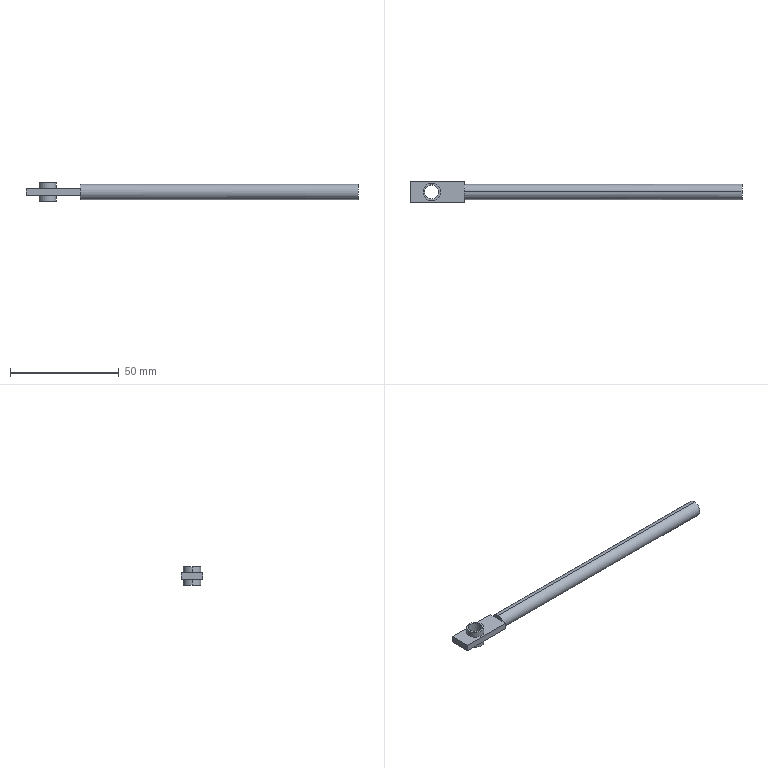Part | STEP file | Gas spring FGS 15089-100 rod | 1 solid | 20 faces | box 153 x 10 x 8.5 mm | volume 5670 mm3 | plane 12 | cylinder 8 | commonest cylinder face diameters 8 x4 6.5 x2 7 x2
STEP:
#1=CARTESIAN_POINT('',(0.,0.,0.));
#2=DIRECTION('',(0.,0.,1.));
#3=DIRECTION('',(1.,0.,0.));
#4=AXIS2_PLACEMENT_3D('',#1,#2,#3);
#5=CARTESIAN_POINT('',(-11.75,0.,-4.25));
#6=VERTEX_POINT('',#5);
#7=CARTESIAN_POINT('',(-11.75,0.,4.25));
#8=VERTEX_POINT('',#7);
#9=CARTESIAN_POINT('',(-11.75,0.,-4.25));
#10=DIRECTION('',(0.,0.,1.));
#11=VECTOR('',#10,1.);
#12=LINE('',#9,#11);
#13=CARTESIAN_POINT('',(-15.,0.,-4.25));
#14=DIRECTION('',(0.,0.,1.));
#15=DIRECTION('',(1.,0.,0.));
#16=AXIS2_PLACEMENT_3D('',#13,#14,#15);
#17=CYLINDRICAL_SURFACE('',#16,3.25);
#18=CARTESIAN_POINT('',(6.283,0.));
#19=DIRECTION('',(0.,1.));
#20=VECTOR('',#19,1.);
#21=LINE('',#18,#20);
#22=(GEOMETRIC_REPRESENTATION_CONTEXT(2)PARAMETRIC_REPRESENTATION_CONTEXT()REPRESENTATION_CONTEXT('',''));
#23=DEFINITIONAL_REPRESENTATION('',(#21),#22);
#24=PCURVE('',#17,#23);
#25=CARTESIAN_POINT('',(-15.,0.,-4.25));
#26=DIRECTION('',(0.,0.,1.));
#27=DIRECTION('',(1.,0.,0.));
#28=AXIS2_PLACEMENT_3D('',#25,#26,#27);
#29=CYLINDRICAL_SURFACE('',#28,3.25);
#30=CARTESIAN_POINT('',(0.,0.));
#31=DIRECTION('',(0.,1.));
#32=VECTOR('',#31,1.);
#33=LINE('',#30,#32);
#34=(GEOMETRIC_REPRESENTATION_CONTEXT(2)PARAMETRIC_REPRESENTATION_CONTEXT()REPRESENTATION_CONTEXT('',''));
#35=DEFINITIONAL_REPRESENTATION('',(#33),#34);
#36=PCURVE('',#29,#35);
#37=SURFACE_CURVE('',#12,(#24,#36),.PCURVE_S1.);
#38=EDGE_CURVE('',#6,#8,#37,.T.);
#39=ORIENTED_EDGE('',*,*,#38,.T.);
#40=CARTESIAN_POINT('',(-18.25,0.,4.25));
#41=VERTEX_POINT('',#40);
#42=CARTESIAN_POINT('',(-15.,0.,4.25));
#43=DIRECTION('',(0.,0.,1.));
#44=DIRECTION('',(1.,0.,0.));
#45=AXIS2_PLACEMENT_3D('',#42,#43,#44);
#46=CIRCLE('',#45,3.25);
#47=CARTESIAN_POINT('',(0.,8.5));
#48=DIRECTION('',(1.,0.));
#49=VECTOR('',#48,1.);
#50=LINE('',#47,#49);
#51=(GEOMETRIC_REPRESENTATION_CONTEXT(2)PARAMETRIC_REPRESENTATION_CONTEXT()REPRESENTATION_CONTEXT('',''));
#52=DEFINITIONAL_REPRESENTATION('',(#50),#51);
#53=PCURVE('',#17,#52);
#54=CARTESIAN_POINT('',(-19.048,-4.048,4.25));
#55=DIRECTION('',(0.,0.,1.));
#56=DIRECTION('',(1.,0.,0.));
#57=AXIS2_PLACEMENT_3D('',#54,#55,#56);
#58=PLANE('',#57);
#59=CARTESIAN_POINT('',(4.048,4.048));
#60=DIRECTION('',(1.,0.));
#61=AXIS2_PLACEMENT_2D('',#59,#60);
#62=CIRCLE('',#61,3.25);
#63=(GEOMETRIC_REPRESENTATION_CONTEXT(2)PARAMETRIC_REPRESENTATION_CONTEXT()REPRESENTATION_CONTEXT('',''));
#64=DEFINITIONAL_REPRESENTATION('',(#62),#63);
#65=PCURVE('',#58,#64);
#66=SURFACE_CURVE('',#46,(#53,#65),.PCURVE_S1.);
#67=EDGE_CURVE('',#41,#8,#66,.T.);
#68=ORIENTED_EDGE('',*,*,#67,.F.);
#69=CARTESIAN_POINT('',(-18.25,0.,-4.25));
#70=VERTEX_POINT('',#69);
#71=CARTESIAN_POINT('',(-18.25,0.,-4.25));
#72=DIRECTION('',(0.,0.,1.));
#73=VECTOR('',#72,1.);
#74=LINE('',#71,#73);
#75=CARTESIAN_POINT('',(3.142,0.));
#76=DIRECTION('',(0.,1.));
#77=VECTOR('',#76,1.);
#78=LINE('',#75,#77);
#79=(GEOMETRIC_REPRESENTATION_CONTEXT(2)PARAMETRIC_REPRESENTATION_CONTEXT()REPRESENTATION_CONTEXT('',''));
#80=DEFINITIONAL_REPRESENTATION('',(#78),#79);
#81=PCURVE('',#17,#80);
#82=CARTESIAN_POINT('',(3.142,0.));
#83=DIRECTION('',(0.,1.));
#84=VECTOR('',#83,1.);
#85=LINE('',#82,#84);
#86=(GEOMETRIC_REPRESENTATION_CONTEXT(2)PARAMETRIC_REPRESENTATION_CONTEXT()REPRESENTATION_CONTEXT('',''));
#87=DEFINITIONAL_REPRESENTATION('',(#85),#86);
#88=PCURVE('',#29,#87);
#89=SURFACE_CURVE('',#74,(#81,#88),.PCURVE_S1.);
#90=EDGE_CURVE('',#70,#41,#89,.T.);
#91=ORIENTED_EDGE('',*,*,#90,.F.);
#92=CARTESIAN_POINT('',(-15.,0.,-4.25));
#93=DIRECTION('',(0.,0.,-1.));
#94=DIRECTION('',(1.,0.,0.));
#95=AXIS2_PLACEMENT_3D('',#92,#93,#94);
#96=CIRCLE('',#95,3.25);
#97=CARTESIAN_POINT('',(6.283,0.));
#98=DIRECTION('',(-1.,0.));
#99=VECTOR('',#98,1.);
#100=LINE('',#97,#99);
#101=(GEOMETRIC_REPRESENTATION_CONTEXT(2)PARAMETRIC_REPRESENTATION_CONTEXT()REPRESENTATION_CONTEXT('',''));
#102=DEFINITIONAL_REPRESENTATION('',(#100),#101);
#103=PCURVE('',#17,#102);
#104=CARTESIAN_POINT('',(-19.048,-4.048,-4.25));
#105=DIRECTION('',(0.,0.,1.));
#106=DIRECTION('',(1.,0.,0.));
#107=AXIS2_PLACEMENT_3D('',#104,#105,#106);
#108=PLANE('',#107);
#109=CARTESIAN_POINT('',(7.298,4.048));
#110=CARTESIAN_POINT('',(7.298,-1.581));
#111=CARTESIAN_POINT('',(2.423,1.233));
#112=CARTESIAN_POINT('',(-2.452,4.048));
#113=CARTESIAN_POINT('',(2.423,6.863));
#114=CARTESIAN_POINT('',(7.298,9.677));
#115=CARTESIAN_POINT('',(7.298,4.048));
#116=(BOUNDED_CURVE()B_SPLINE_CURVE(2,(#109,#110,#111,#112,#113,#114,#115),.UNSPECIFIED.,.T.,.F.)B_SPLINE_CURVE_WITH_KNOTS((1,2,2,2,2,1),(-2.094,0.,2.094,4.189,6.283,8.378),.UNSPECIFIED.)CURVE()GEOMETRIC_REPRESENTATION_ITEM()RATIONAL_B_SPLINE_CURVE((1.,0.5,1.,0.5,1.,0.5,1.))REPRESENTATION_ITEM(''));
#117=(GEOMETRIC_REPRESENTATION_CONTEXT(2)PARAMETRIC_REPRESENTATION_CONTEXT()REPRESENTATION_CONTEXT('',''));
#118=DEFINITIONAL_REPRESENTATION('',(#116),#117);
#119=PCURVE('',#108,#118);
#120=SURFACE_CURVE('',#96,(#103,#119),.PCURVE_S1.);
#121=EDGE_CURVE('',#6,#70,#120,.T.);
#122=ORIENTED_EDGE('',*,*,#121,.F.);
#123=EDGE_LOOP('',(#39,#68,#91,#122));
#124=FACE_BOUND('',#123,.F.);
#125=ADVANCED_FACE('',(#124),#17,.F.);
#126=CARTESIAN_POINT('',(-11.,0.,4.25));
#127=VERTEX_POINT('',#126);
#128=CARTESIAN_POINT('',(-19.,0.,4.25));
#129=VERTEX_POINT('',#128);
#130=CARTESIAN_POINT('',(-15.,0.,4.25));
#131=DIRECTION('',(0.,0.,1.));
#132=DIRECTION('',(-1.,0.,0.));
#133=AXIS2_PLACEMENT_3D('',#130,#131,#132);
#134=CIRCLE('',#133,4.);
#135=CARTESIAN_POINT('',(-15.,0.,4.25));
#136=DIRECTION('',(0.,0.,-1.));
#137=DIRECTION('',(-1.,0.,0.));
#138=AXIS2_PLACEMENT_3D('',#135,#136,#137);
#139=CYLINDRICAL_SURFACE('',#138,4.);
#140=CARTESIAN_POINT('',(6.283,0.));
#141=DIRECTION('',(-1.,0.));
#142=VECTOR('',#141,1.);
#143=LINE('',#140,#142);
#144=(GEOMETRIC_REPRESENTATION_CONTEXT(2)PARAMETRIC_REPRESENTATION_CONTEXT()REPRESENTATION_CONTEXT('',''));
#145=DEFINITIONAL_REPRESENTATION('',(#143),#144);
#146=PCURVE('',#139,#145);
#147=CARTESIAN_POINT('',(4.048,4.048));
#148=DIRECTION('',(-1.,0.));
#149=AXIS2_PLACEMENT_2D('',#147,#148);
#150=CIRCLE('',#149,4.);
#151=(GEOMETRIC_REPRESENTATION_CONTEXT(2)PARAMETRIC_REPRESENTATION_CONTEXT()REPRESENTATION_CONTEXT('',''));
#152=DEFINITIONAL_REPRESENTATION('',(#150),#151);
#153=PCURVE('',#58,#152);
#154=SURFACE_CURVE('',#134,(#146,#153),.PCURVE_S1.);
#155=EDGE_CURVE('',#127,#129,#154,.T.);
#156=ORIENTED_EDGE('',*,*,#155,.F.);
#157=CARTESIAN_POINT('',(-11.,0.,1.5));
#158=VERTEX_POINT('',#157);
#159=CARTESIAN_POINT('',(-11.,0.,4.25));
#160=DIRECTION('',(0.,0.,-1.));
#161=VECTOR('',#160,1.);
#162=LINE('',#159,#161);
#163=CARTESIAN_POINT('',(3.142,0.));
#164=DIRECTION('',(0.,1.));
#165=VECTOR('',#164,1.);
#166=LINE('',#163,#165);
#167=(GEOMETRIC_REPRESENTATION_CONTEXT(2)PARAMETRIC_REPRESENTATION_CONTEXT()REPRESENTATION_CONTEXT('',''));
#168=DEFINITIONAL_REPRESENTATION('',(#166),#167);
#169=PCURVE('',#139,#168);
#170=CARTESIAN_POINT('',(-15.,0.,4.25));
#171=DIRECTION('',(0.,0.,-1.));
#172=DIRECTION('',(-1.,0.,0.));
#173=AXIS2_PLACEMENT_3D('',#170,#171,#172);
#174=CYLINDRICAL_SURFACE('',#173,4.);
#175=CARTESIAN_POINT('',(3.142,0.));
#176=DIRECTION('',(0.,1.));
#177=VECTOR('',#176,1.);
#178=LINE('',#175,#177);
#179=(GEOMETRIC_REPRESENTATION_CONTEXT(2)PARAMETRIC_REPRESENTATION_CONTEXT()REPRESENTATION_CONTEXT('',''));
#180=DEFINITIONAL_REPRESENTATION('',(#178),#179);
#181=PCURVE('',#174,#180);
#182=SURFACE_CURVE('',#162,(#169,#181),.PCURVE_S1.);
#183=EDGE_CURVE('',#127,#158,#182,.T.);
#184=ORIENTED_EDGE('',*,*,#183,.T.);
#185=CARTESIAN_POINT('',(-19.,0.,1.5));
#186=VERTEX_POINT('',#185);
#187=CARTESIAN_POINT('',(-15.,0.,1.5));
#188=DIRECTION('',(0.,0.,-1.));
#189=DIRECTION('',(-1.,0.,0.));
#190=AXIS2_PLACEMENT_3D('',#187,#188,#189);
#191=CIRCLE('',#190,4.);
#192=CARTESIAN_POINT('',(0.,2.75));
#193=DIRECTION('',(1.,0.));
#194=VECTOR('',#193,1.);
#195=LINE('',#192,#194);
#196=(GEOMETRIC_REPRESENTATION_CONTEXT(2)PARAMETRIC_REPRESENTATION_CONTEXT()REPRESENTATION_CONTEXT('',''));
#197=DEFINITIONAL_REPRESENTATION('',(#195),#196);
#198=PCURVE('',#139,#197);
#199=CARTESIAN_POINT('',(0.,-5.,1.5));
#200=DIRECTION('',(0.,0.,-1.));
#201=DIRECTION('',(-1.,0.,0.));
#202=AXIS2_PLACEMENT_3D('',#199,#200,#201);
#203=PLANE('',#202);
#204=CARTESIAN_POINT('',(15.,5.));
#205=DIRECTION('',(1.,0.));
#206=AXIS2_PLACEMENT_2D('',#204,#205);
#207=CIRCLE('',#206,4.);
#208=(GEOMETRIC_REPRESENTATION_CONTEXT(2)PARAMETRIC_REPRESENTATION_CONTEXT()REPRESENTATION_CONTEXT('',''));
#209=DEFINITIONAL_REPRESENTATION('',(#207),#208);
#210=PCURVE('',#203,#209);
#211=SURFACE_CURVE('',#191,(#198,#210),.PCURVE_S1.);
#212=EDGE_CURVE('',#186,#158,#211,.T.);
#213=ORIENTED_EDGE('',*,*,#212,.F.);
#214=CARTESIAN_POINT('',(-19.,0.,4.25));
#215=DIRECTION('',(0.,0.,-1.));
#216=VECTOR('',#215,1.);
#217=LINE('',#214,#216);
#218=CARTESIAN_POINT('',(0.,0.));
#219=DIRECTION('',(0.,1.));
#220=VECTOR('',#219,1.);
#221=LINE('',#218,#220);
#222=(GEOMETRIC_REPRESENTATION_CONTEXT(2)PARAMETRIC_REPRESENTATION_CONTEXT()REPRESENTATION_CONTEXT('',''));
#223=DEFINITIONAL_REPRESENTATION('',(#221),#222);
#224=PCURVE('',#139,#223);
#225=CARTESIAN_POINT('',(6.283,0.));
#226=DIRECTION('',(0.,1.));
#227=VECTOR('',#226,1.);
#228=LINE('',#225,#227);
#229=(GEOMETRIC_REPRESENTATION_CONTEXT(2)PARAMETRIC_REPRESENTATION_CONTEXT()REPRESENTATION_CONTEXT('',''));
#230=DEFINITIONAL_REPRESENTATION('',(#228),#229);
#231=PCURVE('',#174,#230);
#232=SURFACE_CURVE('',#217,(#224,#231),.PCURVE_S1.);
#233=EDGE_CURVE('',#129,#186,#232,.T.);
#234=ORIENTED_EDGE('',*,*,#233,.F.);
#235=EDGE_LOOP('',(#156,#184,#213,#234));
#236=FACE_BOUND('',#235,.T.);
#237=ADVANCED_FACE('',(#236),#139,.T.);
#238=CARTESIAN_POINT('',(-11.,0.,-1.5));
#239=VERTEX_POINT('',#238);
#240=CARTESIAN_POINT('',(-19.,0.,-1.5));
#241=VERTEX_POINT('',#240);
#242=CARTESIAN_POINT('',(-15.,0.,-1.5));
#243=DIRECTION('',(0.,0.,1.));
#244=DIRECTION('',(-1.,0.,0.));
#245=AXIS2_PLACEMENT_3D('',#242,#243,#244);
#246=CIRCLE('',#245,4.);
#247=CARTESIAN_POINT('',(-15.,0.,-1.5));
#248=DIRECTION('',(0.,0.,-1.));
#249=DIRECTION('',(-1.,0.,0.));
#250=AXIS2_PLACEMENT_3D('',#247,#248,#249);
#251=CYLINDRICAL_SURFACE('',#250,4.);
#252=CARTESIAN_POINT('',(6.283,0.));
#253=DIRECTION('',(-1.,0.));
#254=VECTOR('',#253,1.);
#255=LINE('',#252,#254);
#256=(GEOMETRIC_REPRESENTATION_CONTEXT(2)PARAMETRIC_REPRESENTATION_CONTEXT()REPRESENTATION_CONTEXT('',''));
#257=DEFINITIONAL_REPRESENTATION('',(#255),#256);
#258=PCURVE('',#251,#257);
#259=CARTESIAN_POINT('',(-25.,-5.,-1.5));
#260=DIRECTION('',(0.,0.,1.));
#261=DIRECTION('',(1.,0.,0.));
#262=AXIS2_PLACEMENT_3D('',#259,#260,#261);
#263=PLANE('',#262);
#264=CARTESIAN_POINT('',(10.,5.));
#265=DIRECTION('',(-1.,0.));
#266=AXIS2_PLACEMENT_2D('',#264,#265);
#267=CIRCLE('',#266,4.);
#268=(GEOMETRIC_REPRESENTATION_CONTEXT(2)PARAMETRIC_REPRESENTATION_CONTEXT()REPRESENTATION_CONTEXT('',''));
#269=DEFINITIONAL_REPRESENTATION('',(#267),#268);
#270=PCURVE('',#263,#269);
#271=SURFACE_CURVE('',#246,(#258,#270),.PCURVE_S1.);
#272=EDGE_CURVE('',#239,#241,#271,.T.);
#273=ORIENTED_EDGE('',*,*,#272,.F.);
#274=CARTESIAN_POINT('',(-11.,0.,-4.25));
#275=VERTEX_POINT('',#274);
#276=CARTESIAN_POINT('',(-11.,0.,-1.5));
#277=DIRECTION('',(0.,0.,-1.));
#278=VECTOR('',#277,1.);
#279=LINE('',#276,#278);
#280=CARTESIAN_POINT('',(3.142,0.));
#281=DIRECTION('',(0.,1.));
#282=VECTOR('',#281,1.);
#283=LINE('',#280,#282);
#284=(GEOMETRIC_REPRESENTATION_CONTEXT(2)PARAMETRIC_REPRESENTATION_CONTEXT()REPRESENTATION_CONTEXT('',''));
#285=DEFINITIONAL_REPRESENTATION('',(#283),#284);
#286=PCURVE('',#251,#285);
#287=CARTESIAN_POINT('',(-15.,0.,-1.5));
#288=DIRECTION('',(0.,0.,-1.));
#289=DIRECTION('',(-1.,0.,0.));
#290=AXIS2_PLACEMENT_3D('',#287,#288,#289);
#291=CYLINDRICAL_SURFACE('',#290,4.);
#292=CARTESIAN_POINT('',(3.142,0.));
#293=DIRECTION('',(0.,1.));
#294=VECTOR('',#293,1.);
#295=LINE('',#292,#294);
#296=(GEOMETRIC_REPRESENTATION_CONTEXT(2)PARAMETRIC_REPRESENTATION_CONTEXT()REPRESENTATION_CONTEXT('',''));
#297=DEFINITIONAL_REPRESENTATION('',(#295),#296);
#298=PCURVE('',#291,#297);
#299=SURFACE_CURVE('',#279,(#286,#298),.PCURVE_S1.);
#300=EDGE_CURVE('',#239,#275,#299,.T.);
#301=ORIENTED_EDGE('',*,*,#300,.T.);
#302=CARTESIAN_POINT('',(-19.,0.,-4.25));
#303=VERTEX_POINT('',#302);
#304=CARTESIAN_POINT('',(-15.,0.,-4.25));
#305=DIRECTION('',(0.,0.,1.));
#306=DIRECTION('',(-1.,0.,0.));
#307=AXIS2_PLACEMENT_3D('',#304,#305,#306);
#308=CIRCLE('',#307,4.);
#309=CARTESIAN_POINT('',(6.283,2.75));
#310=DIRECTION('',(-1.,0.));
#311=VECTOR('',#310,1.);
#312=LINE('',#309,#311);
#313=(GEOMETRIC_REPRESENTATION_CONTEXT(2)PARAMETRIC_REPRESENTATION_CONTEXT()REPRESENTATION_CONTEXT('',''));
#314=DEFINITIONAL_REPRESENTATION('',(#312),#313);
#315=PCURVE('',#251,#314);
#316=CARTESIAN_POINT('',(4.048,4.048));
#317=DIRECTION('',(-1.,0.));
#318=AXIS2_PLACEMENT_2D('',#316,#317);
#319=CIRCLE('',#318,4.);
#320=(GEOMETRIC_REPRESENTATION_CONTEXT(2)PARAMETRIC_REPRESENTATION_CONTEXT()REPRESENTATION_CONTEXT('',''));
#321=DEFINITIONAL_REPRESENTATION('',(#319),#320);
#322=PCURVE('',#108,#321);
#323=SURFACE_CURVE('',#308,(#315,#322),.PCURVE_S1.);
#324=EDGE_CURVE('',#275,#303,#323,.T.);
#325=ORIENTED_EDGE('',*,*,#324,.T.);
#326=CARTESIAN_POINT('',(-19.,0.,-1.5));
#327=DIRECTION('',(0.,0.,-1.));
#328=VECTOR('',#327,1.);
#329=LINE('',#326,#328);
#330=CARTESIAN_POINT('',(0.,0.));
#331=DIRECTION('',(0.,1.));
#332=VECTOR('',#331,1.);
#333=LINE('',#330,#332);
#334=(GEOMETRIC_REPRESENTATION_CONTEXT(2)PARAMETRIC_REPRESENTATION_CONTEXT()REPRESENTATION_CONTEXT('',''));
#335=DEFINITIONAL_REPRESENTATION('',(#333),#334);
#336=PCURVE('',#251,#335);
#337=CARTESIAN_POINT('',(6.283,0.));
#338=DIRECTION('',(0.,1.));
#339=VECTOR('',#338,1.);
#340=LINE('',#337,#339);
#341=(GEOMETRIC_REPRESENTATION_CONTEXT(2)PARAMETRIC_REPRESENTATION_CONTEXT()REPRESENTATION_CONTEXT('',''));
#342=DEFINITIONAL_REPRESENTATION('',(#340),#341);
#343=PCURVE('',#291,#342);
#344=SURFACE_CURVE('',#329,(#336,#343),.PCURVE_S1.);
#345=EDGE_CURVE('',#241,#303,#344,.T.);
#346=ORIENTED_EDGE('',*,*,#345,.F.);
#347=EDGE_LOOP('',(#273,#301,#325,#346));
#348=FACE_BOUND('',#347,.T.);
#349=ADVANCED_FACE('',(#348),#251,.T.);
#350=CARTESIAN_POINT('',(128.,0.,-3.5));
#351=VERTEX_POINT('',#350);
#352=CARTESIAN_POINT('',(128.,0.,3.5));
#353=VERTEX_POINT('',#352);
#354=CARTESIAN_POINT('',(128.,0.,0.));
#355=DIRECTION('',(1.,0.,0.));
#356=DIRECTION('',(0.,0.,1.));
#357=AXIS2_PLACEMENT_3D('',#354,#355,#356);
#358=CIRCLE('',#357,3.5);
#359=CARTESIAN_POINT('',(128.,0.,0.));
#360=DIRECTION('',(-1.,0.,0.));
#361=DIRECTION('',(0.,0.,1.));
#362=AXIS2_PLACEMENT_3D('',#359,#360,#361);
#363=CYLINDRICAL_SURFACE('',#362,3.5);
#364=CARTESIAN_POINT('',(6.283,0.));
#365=DIRECTION('',(-1.,0.));
#366=VECTOR('',#365,1.);
#367=LINE('',#364,#366);
#368=(GEOMETRIC_REPRESENTATION_CONTEXT(2)PARAMETRIC_REPRESENTATION_CONTEXT()REPRESENTATION_CONTEXT('',''));
#369=DEFINITIONAL_REPRESENTATION('',(#367),#368);
#370=PCURVE('',#363,#369);
#371=CARTESIAN_POINT('',(128.,-3.542,3.542));
#372=DIRECTION('',(1.,0.,0.));
#373=DIRECTION('',(0.,0.,-1.));
#374=AXIS2_PLACEMENT_3D('',#371,#372,#373);
#375=PLANE('',#374);
#376=CARTESIAN_POINT('',(3.542,3.542));
#377=DIRECTION('',(-1.,0.));
#378=AXIS2_PLACEMENT_2D('',#376,#377);
#379=CIRCLE('',#378,3.5);
#380=(GEOMETRIC_REPRESENTATION_CONTEXT(2)PARAMETRIC_REPRESENTATION_CONTEXT()REPRESENTATION_CONTEXT('',''));
#381=DEFINITIONAL_REPRESENTATION('',(#379),#380);
#382=PCURVE('',#375,#381);
#383=SURFACE_CURVE('',#358,(#370,#382),.PCURVE_S1.);
#384=EDGE_CURVE('',#351,#353,#383,.T.);
#385=ORIENTED_EDGE('',*,*,#384,.F.);
#386=CARTESIAN_POINT('',(0.,0.,-3.5));
#387=VERTEX_POINT('',#386);
#388=CARTESIAN_POINT('',(128.,0.,-3.5));
#389=DIRECTION('',(-1.,0.,0.));
#390=VECTOR('',#389,1.);
#391=LINE('',#388,#390);
#392=CARTESIAN_POINT('',(3.142,0.));
#393=DIRECTION('',(0.,1.));
#394=VECTOR('',#393,1.);
#395=LINE('',#392,#394);
#396=(GEOMETRIC_REPRESENTATION_CONTEXT(2)PARAMETRIC_REPRESENTATION_CONTEXT()REPRESENTATION_CONTEXT('',''));
#397=DEFINITIONAL_REPRESENTATION('',(#395),#396);
#398=PCURVE('',#363,#397);
#399=CARTESIAN_POINT('',(128.,0.,0.));
#400=DIRECTION('',(-1.,0.,0.));
#401=DIRECTION('',(0.,0.,1.));
#402=AXIS2_PLACEMENT_3D('',#399,#400,#401);
#403=CYLINDRICAL_SURFACE('',#402,3.5);
#404=CARTESIAN_POINT('',(3.142,0.));
#405=DIRECTION('',(0.,1.));
#406=VECTOR('',#405,1.);
#407=LINE('',#404,#406);
#408=(GEOMETRIC_REPRESENTATION_CONTEXT(2)PARAMETRIC_REPRESENTATION_CONTEXT()REPRESENTATION_CONTEXT('',''));
#409=DEFINITIONAL_REPRESENTATION('',(#407),#408);
#410=PCURVE('',#403,#409);
#411=SURFACE_CURVE('',#391,(#398,#410),.PCURVE_S1.);
#412=EDGE_CURVE('',#351,#387,#411,.T.);
#413=ORIENTED_EDGE('',*,*,#412,.T.);
#414=CARTESIAN_POINT('',(0.,3.162,-1.5));
#415=VERTEX_POINT('',#414);
#416=CARTESIAN_POINT('',(0.,0.,0.));
#417=DIRECTION('',(1.,0.,0.));
#418=DIRECTION('',(0.,0.,1.));
#419=AXIS2_PLACEMENT_3D('',#416,#417,#418);
#420=CIRCLE('',#419,3.5);
#421=CARTESIAN_POINT('',(6.283,128.));
#422=DIRECTION('',(-1.,0.));
#423=VECTOR('',#422,1.);
#424=LINE('',#421,#423);
#425=(GEOMETRIC_REPRESENTATION_CONTEXT(2)PARAMETRIC_REPRESENTATION_CONTEXT()REPRESENTATION_CONTEXT('',''));
#426=DEFINITIONAL_REPRESENTATION('',(#424),#425);
#427=PCURVE('',#363,#426);
#428=CARTESIAN_POINT('',(0.,-3.2,-1.5));
#429=DIRECTION('',(1.,0.,0.));
#430=DIRECTION('',(0.,0.,-1.));
#431=AXIS2_PLACEMENT_3D('',#428,#429,#430);
#432=PLANE('',#431);
#433=CARTESIAN_POINT('',(-1.5,3.2));
#434=DIRECTION('',(-1.,0.));
#435=AXIS2_PLACEMENT_2D('',#433,#434);
#436=CIRCLE('',#435,3.5);
#437=(GEOMETRIC_REPRESENTATION_CONTEXT(2)PARAMETRIC_REPRESENTATION_CONTEXT()REPRESENTATION_CONTEXT('',''));
#438=DEFINITIONAL_REPRESENTATION('',(#436),#437);
#439=PCURVE('',#432,#438);
#440=SURFACE_CURVE('',#420,(#427,#439),.PCURVE_S1.);
#441=EDGE_CURVE('',#387,#415,#440,.T.);
#442=ORIENTED_EDGE('',*,*,#441,.T.);
#443=CARTESIAN_POINT('',(0.,3.162,1.5));
#444=VERTEX_POINT('',#443);
#445=CARTESIAN_POINT('',(0.,0.,0.));
#446=DIRECTION('',(1.,0.,0.));
#447=DIRECTION('',(0.,0.,1.));
#448=AXIS2_PLACEMENT_3D('',#445,#446,#447);
#449=CIRCLE('',#448,3.5);
#450=CARTESIAN_POINT('',(6.283,128.));
#451=DIRECTION('',(-1.,0.));
#452=VECTOR('',#451,1.);
#453=LINE('',#450,#452);
#454=(GEOMETRIC_REPRESENTATION_CONTEXT(2)PARAMETRIC_REPRESENTATION_CONTEXT()REPRESENTATION_CONTEXT('',''));
#455=DEFINITIONAL_REPRESENTATION('',(#453),#454);
#456=PCURVE('',#363,#455);
#457=CARTESIAN_POINT('',(0.,3.151,-1.5));
#458=DIRECTION('',(-1.,0.,0.));
#459=DIRECTION('',(0.,0.,1.));
#460=AXIS2_PLACEMENT_3D('',#457,#458,#459);
#461=PLANE('',#460);
#462=CARTESIAN_POINT('',(5.,-3.151));
#463=CARTESIAN_POINT('',(5.,-9.213));
#464=CARTESIAN_POINT('',(-0.25,-6.182));
#465=CARTESIAN_POINT('',(-5.5,-3.151));
#466=CARTESIAN_POINT('',(-0.25,-0.1202));
#467=CARTESIAN_POINT('',(5.,2.911));
#468=CARTESIAN_POINT('',(5.,-3.151));
#469=(BOUNDED_CURVE()B_SPLINE_CURVE(2,(#462,#463,#464,#465,#466,#467,#468),.UNSPECIFIED.,.T.,.F.)B_SPLINE_CURVE_WITH_KNOTS((1,2,2,2,2,1),(-2.094,0.,2.094,4.189,6.283,8.378),.UNSPECIFIED.)CURVE()GEOMETRIC_REPRESENTATION_ITEM()RATIONAL_B_SPLINE_CURVE((1.,0.5,1.,0.5,1.,0.5,1.))REPRESENTATION_ITEM(''));
#470=(GEOMETRIC_REPRESENTATION_CONTEXT(2)PARAMETRIC_REPRESENTATION_CONTEXT()REPRESENTATION_CONTEXT('',''));
#471=DEFINITIONAL_REPRESENTATION('',(#469),#470);
#472=PCURVE('',#461,#471);
#473=SURFACE_CURVE('',#449,(#456,#472),.PCURVE_S1.);
#474=EDGE_CURVE('',#415,#444,#473,.T.);
#475=ORIENTED_EDGE('',*,*,#474,.T.);
#476=CARTESIAN_POINT('',(0.,0.,3.5));
#477=VERTEX_POINT('',#476);
#478=CARTESIAN_POINT('',(0.,0.,0.));
#479=DIRECTION('',(1.,0.,0.));
#480=DIRECTION('',(0.,0.,1.));
#481=AXIS2_PLACEMENT_3D('',#478,#479,#480);
#482=CIRCLE('',#481,3.5);
#483=CARTESIAN_POINT('',(6.283,128.));
#484=DIRECTION('',(-1.,0.));
#485=VECTOR('',#484,1.);
#486=LINE('',#483,#485);
#487=(GEOMETRIC_REPRESENTATION_CONTEXT(2)PARAMETRIC_REPRESENTATION_CONTEXT()REPRESENTATION_CONTEXT('',''));
#488=DEFINITIONAL_REPRESENTATION('',(#486),#487);
#489=PCURVE('',#363,#488);
#490=CARTESIAN_POINT('',(0.,-3.2,3.512));
#491=DIRECTION('',(1.,0.,0.));
#492=DIRECTION('',(0.,0.,-1.));
#493=AXIS2_PLACEMENT_3D('',#490,#491,#492);
#494=PLANE('',#493);
#495=CARTESIAN_POINT('',(3.512,3.2));
#496=DIRECTION('',(-1.,0.));
#497=AXIS2_PLACEMENT_2D('',#495,#496);
#498=CIRCLE('',#497,3.5);
#499=(GEOMETRIC_REPRESENTATION_CONTEXT(2)PARAMETRIC_REPRESENTATION_CONTEXT()REPRESENTATION_CONTEXT('',''));
#500=DEFINITIONAL_REPRESENTATION('',(#498),#499);
#501=PCURVE('',#494,#500);
#502=SURFACE_CURVE('',#482,(#489,#501),.PCURVE_S1.);
#503=EDGE_CURVE('',#444,#477,#502,.T.);
#504=ORIENTED_EDGE('',*,*,#503,.T.);
#505=CARTESIAN_POINT('',(128.,0.,3.5));
#506=DIRECTION('',(-1.,0.,0.));
#507=VECTOR('',#506,1.);
#508=LINE('',#505,#507);
#509=CARTESIAN_POINT('',(0.,0.));
#510=DIRECTION('',(0.,1.));
#511=VECTOR('',#510,1.);
#512=LINE('',#509,#511);
#513=(GEOMETRIC_REPRESENTATION_CONTEXT(2)PARAMETRIC_REPRESENTATION_CONTEXT()REPRESENTATION_CONTEXT('',''));
#514=DEFINITIONAL_REPRESENTATION('',(#512),#513);
#515=PCURVE('',#363,#514);
#516=CARTESIAN_POINT('',(6.283,0.));
#517=DIRECTION('',(0.,1.));
#518=VECTOR('',#517,1.);
#519=LINE('',#516,#518);
#520=(GEOMETRIC_REPRESENTATION_CONTEXT(2)PARAMETRIC_REPRESENTATION_CONTEXT()REPRESENTATION_CONTEXT('',''));
#521=DEFINITIONAL_REPRESENTATION('',(#519),#520);
#522=PCURVE('',#403,#521);
#523=SURFACE_CURVE('',#508,(#515,#522),.PCURVE_S1.);
#524=EDGE_CURVE('',#353,#477,#523,.T.);
#525=ORIENTED_EDGE('',*,*,#524,.F.);
#526=EDGE_LOOP('',(#385,#413,#442,#475,#504,#525));
#527=FACE_BOUND('',#526,.T.);
#528=ADVANCED_FACE('',(#527),#363,.T.);
#529=CARTESIAN_POINT('',(-15.,0.,4.25));
#530=DIRECTION('',(0.,0.,1.));
#531=DIRECTION('',(1.,0.,0.));
#532=AXIS2_PLACEMENT_3D('',#529,#530,#531);
#533=CIRCLE('',#532,3.25);
#534=CARTESIAN_POINT('',(0.,8.5));
#535=DIRECTION('',(1.,0.));
#536=VECTOR('',#535,1.);
#537=LINE('',#534,#536);
#538=(GEOMETRIC_REPRESENTATION_CONTEXT(2)PARAMETRIC_REPRESENTATION_CONTEXT()REPRESENTATION_CONTEXT('',''));
#539=DEFINITIONAL_REPRESENTATION('',(#537),#538);
#540=PCURVE('',#29,#539);
#541=CARTESIAN_POINT('',(4.048,4.048));
#542=DIRECTION('',(1.,0.));
#543=AXIS2_PLACEMENT_2D('',#541,#542);
#544=CIRCLE('',#543,3.25);
#545=(GEOMETRIC_REPRESENTATION_CONTEXT(2)PARAMETRIC_REPRESENTATION_CONTEXT()REPRESENTATION_CONTEXT('',''));
#546=DEFINITIONAL_REPRESENTATION('',(#544),#545);
#547=PCURVE('',#58,#546);
#548=SURFACE_CURVE('',#533,(#540,#547),.PCURVE_S1.);
#549=EDGE_CURVE('',#8,#41,#548,.T.);
#550=ORIENTED_EDGE('',*,*,#549,.F.);
#551=ORIENTED_EDGE('',*,*,#38,.F.);
#552=CARTESIAN_POINT('',(-15.,0.,-4.25));
#553=DIRECTION('',(0.,0.,-1.));
#554=DIRECTION('',(1.,0.,0.));
#555=AXIS2_PLACEMENT_3D('',#552,#553,#554);
#556=CIRCLE('',#555,3.25);
#557=CARTESIAN_POINT('',(6.283,0.));
#558=DIRECTION('',(-1.,0.));
#559=VECTOR('',#558,1.);
#560=LINE('',#557,#559);
#561=(GEOMETRIC_REPRESENTATION_CONTEXT(2)PARAMETRIC_REPRESENTATION_CONTEXT()REPRESENTATION_CONTEXT('',''));
#562=DEFINITIONAL_REPRESENTATION('',(#560),#561);
#563=PCURVE('',#29,#562);
#564=CARTESIAN_POINT('',(7.298,4.048));
#565=CARTESIAN_POINT('',(7.298,-1.581));
#566=CARTESIAN_POINT('',(2.423,1.233));
#567=CARTESIAN_POINT('',(-2.452,4.048));
#568=CARTESIAN_POINT('',(2.423,6.863));
#569=CARTESIAN_POINT('',(7.298,9.677));
#570=CARTESIAN_POINT('',(7.298,4.048));
#571=(BOUNDED_CURVE()B_SPLINE_CURVE(2,(#564,#565,#566,#567,#568,#569,#570),.UNSPECIFIED.,.T.,.F.)B_SPLINE_CURVE_WITH_KNOTS((1,2,2,2,2,1),(-2.094,0.,2.094,4.189,6.283,8.378),.UNSPECIFIED.)CURVE()GEOMETRIC_REPRESENTATION_ITEM()RATIONAL_B_SPLINE_CURVE((1.,0.5,1.,0.5,1.,0.5,1.))REPRESENTATION_ITEM(''));
#572=(GEOMETRIC_REPRESENTATION_CONTEXT(2)PARAMETRIC_REPRESENTATION_CONTEXT()REPRESENTATION_CONTEXT('',''));
#573=DEFINITIONAL_REPRESENTATION('',(#571),#572);
#574=PCURVE('',#108,#573);
#575=SURFACE_CURVE('',#556,(#563,#574),.PCURVE_S1.);
#576=EDGE_CURVE('',#70,#6,#575,.T.);
#577=ORIENTED_EDGE('',*,*,#576,.F.);
#578=ORIENTED_EDGE('',*,*,#90,.T.);
#579=EDGE_LOOP('',(#550,#551,#577,#578));
#580=FACE_BOUND('',#579,.F.);
#581=ADVANCED_FACE('',(#580),#29,.F.);
#582=ORIENTED_EDGE('',*,*,#549,.F.);
#583=ORIENTED_EDGE('',*,*,#67,.F.);
#584=EDGE_LOOP('',(#582,#583));
#585=FACE_BOUND('',#584,.T.);
#586=CARTESIAN_POINT('',(-15.,0.,4.25));
#587=DIRECTION('',(0.,0.,1.));
#588=DIRECTION('',(-1.,0.,0.));
#589=AXIS2_PLACEMENT_3D('',#586,#587,#588);
#590=CIRCLE('',#589,4.);
#591=CARTESIAN_POINT('',(4.048,4.048));
#592=DIRECTION('',(-1.,0.));
#593=AXIS2_PLACEMENT_2D('',#591,#592);
#594=CIRCLE('',#593,4.);
#595=(GEOMETRIC_REPRESENTATION_CONTEXT(2)PARAMETRIC_REPRESENTATION_CONTEXT()REPRESENTATION_CONTEXT('',''));
#596=DEFINITIONAL_REPRESENTATION('',(#594),#595);
#597=PCURVE('',#58,#596);
#598=CARTESIAN_POINT('',(6.283,0.));
#599=DIRECTION('',(-1.,0.));
#600=VECTOR('',#599,1.);
#601=LINE('',#598,#600);
#602=(GEOMETRIC_REPRESENTATION_CONTEXT(2)PARAMETRIC_REPRESENTATION_CONTEXT()REPRESENTATION_CONTEXT('',''));
#603=DEFINITIONAL_REPRESENTATION('',(#601),#602);
#604=PCURVE('',#174,#603);
#605=SURFACE_CURVE('',#590,(#597,#604),.PCURVE_S1.);
#606=EDGE_CURVE('',#129,#127,#605,.T.);
#607=ORIENTED_EDGE('',*,*,#606,.T.);
#608=ORIENTED_EDGE('',*,*,#155,.T.);
#609=EDGE_LOOP('',(#607,#608));
#610=FACE_BOUND('',#609,.T.);
#611=ADVANCED_FACE('',(#585,#610),#58,.T.);
#612=ORIENTED_EDGE('',*,*,#121,.F.);
#613=ORIENTED_EDGE('',*,*,#576,.F.);
#614=EDGE_LOOP('',(#612,#613));
#615=FACE_BOUND('',#614,.T.);
#616=CARTESIAN_POINT('',(-15.,0.,-4.25));
#617=DIRECTION('',(0.,0.,1.));
#618=DIRECTION('',(-1.,0.,0.));
#619=AXIS2_PLACEMENT_3D('',#616,#617,#618);
#620=CIRCLE('',#619,4.);
#621=CARTESIAN_POINT('',(4.048,4.048));
#622=DIRECTION('',(-1.,0.));
#623=AXIS2_PLACEMENT_2D('',#621,#622);
#624=CIRCLE('',#623,4.);
#625=(GEOMETRIC_REPRESENTATION_CONTEXT(2)PARAMETRIC_REPRESENTATION_CONTEXT()REPRESENTATION_CONTEXT('',''));
#626=DEFINITIONAL_REPRESENTATION('',(#624),#625);
#627=PCURVE('',#108,#626);
#628=CARTESIAN_POINT('',(6.283,2.75));
#629=DIRECTION('',(-1.,0.));
#630=VECTOR('',#629,1.);
#631=LINE('',#628,#630);
#632=(GEOMETRIC_REPRESENTATION_CONTEXT(2)PARAMETRIC_REPRESENTATION_CONTEXT()REPRESENTATION_CONTEXT('',''));
#633=DEFINITIONAL_REPRESENTATION('',(#631),#632);
#634=PCURVE('',#291,#633);
#635=SURFACE_CURVE('',#620,(#627,#634),.PCURVE_S1.);
#636=EDGE_CURVE('',#303,#275,#635,.T.);
#637=ORIENTED_EDGE('',*,*,#636,.F.);
#638=ORIENTED_EDGE('',*,*,#324,.F.);
#639=EDGE_LOOP('',(#637,#638));
#640=FACE_BOUND('',#639,.T.);
#641=ADVANCED_FACE('',(#615,#640),#108,.F.);
#642=ORIENTED_EDGE('',*,*,#183,.F.);
#643=ORIENTED_EDGE('',*,*,#606,.F.);
#644=ORIENTED_EDGE('',*,*,#233,.T.);
#645=CARTESIAN_POINT('',(-15.,0.,1.5));
#646=DIRECTION('',(0.,0.,-1.));
#647=DIRECTION('',(-1.,0.,0.));
#648=AXIS2_PLACEMENT_3D('',#645,#646,#647);
#649=CIRCLE('',#648,4.);
#650=CARTESIAN_POINT('',(0.,2.75));
#651=DIRECTION('',(1.,0.));
#652=VECTOR('',#651,1.);
#653=LINE('',#650,#652);
#654=(GEOMETRIC_REPRESENTATION_CONTEXT(2)PARAMETRIC_REPRESENTATION_CONTEXT()REPRESENTATION_CONTEXT('',''));
#655=DEFINITIONAL_REPRESENTATION('',(#653),#654);
#656=PCURVE('',#174,#655);
#657=CARTESIAN_POINT('',(15.,5.));
#658=DIRECTION('',(1.,0.));
#659=AXIS2_PLACEMENT_2D('',#657,#658);
#660=CIRCLE('',#659,4.);
#661=(GEOMETRIC_REPRESENTATION_CONTEXT(2)PARAMETRIC_REPRESENTATION_CONTEXT()REPRESENTATION_CONTEXT('',''));
#662=DEFINITIONAL_REPRESENTATION('',(#660),#661);
#663=PCURVE('',#203,#662);
#664=SURFACE_CURVE('',#649,(#656,#663),.PCURVE_S1.);
#665=EDGE_CURVE('',#158,#186,#664,.T.);
#666=ORIENTED_EDGE('',*,*,#665,.F.);
#667=EDGE_LOOP('',(#642,#643,#644,#666));
#668=FACE_BOUND('',#667,.T.);
#669=ADVANCED_FACE('',(#668),#174,.T.);
#670=ORIENTED_EDGE('',*,*,#300,.F.);
#671=CARTESIAN_POINT('',(-15.,0.,-1.5));
#672=DIRECTION('',(0.,0.,1.));
#673=DIRECTION('',(-1.,0.,0.));
#674=AXIS2_PLACEMENT_3D('',#671,#672,#673);
#675=CIRCLE('',#674,4.);
#676=CARTESIAN_POINT('',(6.283,0.));
#677=DIRECTION('',(-1.,0.));
#678=VECTOR('',#677,1.);
#679=LINE('',#676,#678);
#680=(GEOMETRIC_REPRESENTATION_CONTEXT(2)PARAMETRIC_REPRESENTATION_CONTEXT()REPRESENTATION_CONTEXT('',''));
#681=DEFINITIONAL_REPRESENTATION('',(#679),#680);
#682=PCURVE('',#291,#681);
#683=CARTESIAN_POINT('',(10.,5.));
#684=DIRECTION('',(-1.,0.));
#685=AXIS2_PLACEMENT_2D('',#683,#684);
#686=CIRCLE('',#685,4.);
#687=(GEOMETRIC_REPRESENTATION_CONTEXT(2)PARAMETRIC_REPRESENTATION_CONTEXT()REPRESENTATION_CONTEXT('',''));
#688=DEFINITIONAL_REPRESENTATION('',(#686),#687);
#689=PCURVE('',#263,#688);
#690=SURFACE_CURVE('',#675,(#682,#689),.PCURVE_S1.);
#691=EDGE_CURVE('',#241,#239,#690,.T.);
#692=ORIENTED_EDGE('',*,*,#691,.F.);
#693=ORIENTED_EDGE('',*,*,#345,.T.);
#694=ORIENTED_EDGE('',*,*,#636,.T.);
#695=EDGE_LOOP('',(#670,#692,#693,#694));
#696=FACE_BOUND('',#695,.T.);
#697=ADVANCED_FACE('',(#696),#291,.T.);
#698=ORIENTED_EDGE('',*,*,#212,.T.);
#699=ORIENTED_EDGE('',*,*,#665,.T.);
#700=EDGE_LOOP('',(#698,#699));
#701=FACE_BOUND('',#700,.T.);
#702=CARTESIAN_POINT('',(0.,-3.162,1.5));
#703=VERTEX_POINT('',#702);
#704=CARTESIAN_POINT('',(0.,-5.,1.5));
#705=VERTEX_POINT('',#704);
#706=CARTESIAN_POINT('',(0.,0.,1.5));
#707=DIRECTION('',(0.,-1.,0.));
#708=VECTOR('',#707,1.);
#709=LINE('',#706,#708);
#710=CARTESIAN_POINT('',(0.,5.));
#711=DIRECTION('',(0.,-1.));
#712=VECTOR('',#711,1.);
#713=LINE('',#710,#712);
#714=(GEOMETRIC_REPRESENTATION_CONTEXT(2)PARAMETRIC_REPRESENTATION_CONTEXT()REPRESENTATION_CONTEXT('',''));
#715=DEFINITIONAL_REPRESENTATION('',(#713),#714);
#716=PCURVE('',#203,#715);
#717=CARTESIAN_POINT('',(0.,-5.,-1.5));
#718=DIRECTION('',(-1.,0.,0.));
#719=DIRECTION('',(0.,0.,1.));
#720=AXIS2_PLACEMENT_3D('',#717,#718,#719);
#721=PLANE('',#720);
#722=CARTESIAN_POINT('',(3.,5.));
#723=DIRECTION('',(0.,-1.));
#724=VECTOR('',#723,1.);
#725=LINE('',#722,#724);
#726=(GEOMETRIC_REPRESENTATION_CONTEXT(2)PARAMETRIC_REPRESENTATION_CONTEXT()REPRESENTATION_CONTEXT('',''));
#727=DEFINITIONAL_REPRESENTATION('',(#725),#726);
#728=PCURVE('',#721,#727);
#729=SURFACE_CURVE('',#709,(#716,#728),.PCURVE_S1.);
#730=EDGE_CURVE('',#703,#705,#729,.T.);
#731=ORIENTED_EDGE('',*,*,#730,.F.);
#732=CARTESIAN_POINT('',(0.,0.,1.5));
#733=DIRECTION('',(0.,-1.,0.));
#734=VECTOR('',#733,1.);
#735=LINE('',#732,#734);
#736=CARTESIAN_POINT('',(0.,5.));
#737=DIRECTION('',(0.,-1.));
#738=VECTOR('',#737,1.);
#739=LINE('',#736,#738);
#740=(GEOMETRIC_REPRESENTATION_CONTEXT(2)PARAMETRIC_REPRESENTATION_CONTEXT()REPRESENTATION_CONTEXT('',''));
#741=DEFINITIONAL_REPRESENTATION('',(#739),#740);
#742=PCURVE('',#203,#741);
#743=CARTESIAN_POINT('',(2.012,3.2));
#744=DIRECTION('',(0.,-1.));
#745=VECTOR('',#744,1.);
#746=LINE('',#743,#745);
#747=(GEOMETRIC_REPRESENTATION_CONTEXT(2)PARAMETRIC_REPRESENTATION_CONTEXT()REPRESENTATION_CONTEXT('',''));
#748=DEFINITIONAL_REPRESENTATION('',(#746),#747);
#749=PCURVE('',#494,#748);
#750=SURFACE_CURVE('',#735,(#742,#749),.PCURVE_S1.);
#751=EDGE_CURVE('',#444,#703,#750,.T.);
#752=ORIENTED_EDGE('',*,*,#751,.F.);
#753=CARTESIAN_POINT('',(0.,5.,1.5));
#754=VERTEX_POINT('',#753);
#755=CARTESIAN_POINT('',(0.,0.,1.5));
#756=DIRECTION('',(0.,-1.,0.));
#757=VECTOR('',#756,1.);
#758=LINE('',#755,#757);
#759=CARTESIAN_POINT('',(0.,5.));
#760=DIRECTION('',(0.,-1.));
#761=VECTOR('',#760,1.);
#762=LINE('',#759,#761);
#763=(GEOMETRIC_REPRESENTATION_CONTEXT(2)PARAMETRIC_REPRESENTATION_CONTEXT()REPRESENTATION_CONTEXT('',''));
#764=DEFINITIONAL_REPRESENTATION('',(#762),#763);
#765=PCURVE('',#203,#764);
#766=CARTESIAN_POINT('',(3.,-3.151));
#767=DIRECTION('',(0.,-1.));
#768=VECTOR('',#767,1.);
#769=LINE('',#766,#768);
#770=(GEOMETRIC_REPRESENTATION_CONTEXT(2)PARAMETRIC_REPRESENTATION_CONTEXT()REPRESENTATION_CONTEXT('',''));
#771=DEFINITIONAL_REPRESENTATION('',(#769),#770);
#772=PCURVE('',#461,#771);
#773=SURFACE_CURVE('',#758,(#765,#772),.PCURVE_S1.);
#774=EDGE_CURVE('',#754,#444,#773,.T.);
#775=ORIENTED_EDGE('',*,*,#774,.F.);
#776=CARTESIAN_POINT('',(-25.,5.,1.5));
#777=VERTEX_POINT('',#776);
#778=CARTESIAN_POINT('',(-12.5,5.,1.5));
#779=DIRECTION('',(1.,0.,0.));
#780=VECTOR('',#779,1.);
#781=LINE('',#778,#780);
#782=CARTESIAN_POINT('',(12.5,10.));
#783=DIRECTION('',(-1.,0.));
#784=VECTOR('',#783,1.);
#785=LINE('',#782,#784);
#786=(GEOMETRIC_REPRESENTATION_CONTEXT(2)PARAMETRIC_REPRESENTATION_CONTEXT()REPRESENTATION_CONTEXT('',''));
#787=DEFINITIONAL_REPRESENTATION('',(#785),#786);
#788=PCURVE('',#203,#787);
#789=CARTESIAN_POINT('',(-25.,5.,1.5));
#790=DIRECTION('',(0.,-1.,0.));
#791=DIRECTION('',(0.,0.,-1.));
#792=AXIS2_PLACEMENT_3D('',#789,#790,#791);
#793=PLANE('',#792);
#794=CARTESIAN_POINT('',(0.,12.5));
#795=DIRECTION('',(0.,1.));
#796=VECTOR('',#795,1.);
#797=LINE('',#794,#796);
#798=(GEOMETRIC_REPRESENTATION_CONTEXT(2)PARAMETRIC_REPRESENTATION_CONTEXT()REPRESENTATION_CONTEXT('',''));
#799=DEFINITIONAL_REPRESENTATION('',(#797),#798);
#800=PCURVE('',#793,#799);
#801=SURFACE_CURVE('',#781,(#788,#800),.PCURVE_S1.);
#802=EDGE_CURVE('',#777,#754,#801,.T.);
#803=ORIENTED_EDGE('',*,*,#802,.F.);
#804=CARTESIAN_POINT('',(-25.,-5.,1.5));
#805=VERTEX_POINT('',#804);
#806=CARTESIAN_POINT('',(-25.,0.,1.5));
#807=DIRECTION('',(0.,1.,0.));
#808=VECTOR('',#807,1.);
#809=LINE('',#806,#808);
#810=CARTESIAN_POINT('',(25.,5.));
#811=DIRECTION('',(0.,1.));
#812=VECTOR('',#811,1.);
#813=LINE('',#810,#812);
#814=(GEOMETRIC_REPRESENTATION_CONTEXT(2)PARAMETRIC_REPRESENTATION_CONTEXT()REPRESENTATION_CONTEXT('',''));
#815=DEFINITIONAL_REPRESENTATION('',(#813),#814);
#816=PCURVE('',#203,#815);
#817=CARTESIAN_POINT('',(-25.,-5.,1.5));
#818=DIRECTION('',(1.,0.,0.));
#819=DIRECTION('',(0.,0.,-1.));
#820=AXIS2_PLACEMENT_3D('',#817,#818,#819);
#821=PLANE('',#820);
#822=CARTESIAN_POINT('',(0.,5.));
#823=DIRECTION('',(0.,1.));
#824=VECTOR('',#823,1.);
#825=LINE('',#822,#824);
#826=(GEOMETRIC_REPRESENTATION_CONTEXT(2)PARAMETRIC_REPRESENTATION_CONTEXT()REPRESENTATION_CONTEXT('',''));
#827=DEFINITIONAL_REPRESENTATION('',(#825),#826);
#828=PCURVE('',#821,#827);
#829=SURFACE_CURVE('',#809,(#816,#828),.PCURVE_S1.);
#830=EDGE_CURVE('',#805,#777,#829,.T.);
#831=ORIENTED_EDGE('',*,*,#830,.F.);
#832=CARTESIAN_POINT('',(-12.5,-5.,1.5));
#833=DIRECTION('',(-1.,0.,0.));
#834=VECTOR('',#833,1.);
#835=LINE('',#832,#834);
#836=CARTESIAN_POINT('',(12.5,0.));
#837=DIRECTION('',(1.,0.));
#838=VECTOR('',#837,1.);
#839=LINE('',#836,#838);
#840=(GEOMETRIC_REPRESENTATION_CONTEXT(2)PARAMETRIC_REPRESENTATION_CONTEXT()REPRESENTATION_CONTEXT('',''));
#841=DEFINITIONAL_REPRESENTATION('',(#839),#840);
#842=PCURVE('',#203,#841);
#843=CARTESIAN_POINT('',(-25.,-5.,1.5));
#844=DIRECTION('',(0.,-1.,0.));
#845=DIRECTION('',(0.,0.,-1.));
#846=AXIS2_PLACEMENT_3D('',#843,#844,#845);
#847=PLANE('',#846);
#848=CARTESIAN_POINT('',(0.,12.5));
#849=DIRECTION('',(0.,-1.));
#850=VECTOR('',#849,1.);
#851=LINE('',#848,#850);
#852=(GEOMETRIC_REPRESENTATION_CONTEXT(2)PARAMETRIC_REPRESENTATION_CONTEXT()REPRESENTATION_CONTEXT('',''));
#853=DEFINITIONAL_REPRESENTATION('',(#851),#852);
#854=PCURVE('',#847,#853);
#855=SURFACE_CURVE('',#835,(#842,#854),.PCURVE_S1.);
#856=EDGE_CURVE('',#705,#805,#855,.T.);
#857=ORIENTED_EDGE('',*,*,#856,.F.);
#858=EDGE_LOOP('',(#731,#752,#775,#803,#831,#857));
#859=FACE_BOUND('',#858,.T.);
#860=ADVANCED_FACE('',(#701,#859),#203,.F.);
#861=ORIENTED_EDGE('',*,*,#691,.T.);
#862=ORIENTED_EDGE('',*,*,#272,.T.);
#863=EDGE_LOOP('',(#861,#862));
#864=FACE_BOUND('',#863,.T.);
#865=CARTESIAN_POINT('',(-25.,5.,-1.5));
#866=VERTEX_POINT('',#865);
#867=CARTESIAN_POINT('',(-25.,-5.,-1.5));
#868=VERTEX_POINT('',#867);
#869=CARTESIAN_POINT('',(-25.,0.,-1.5));
#870=DIRECTION('',(0.,-1.,0.));
#871=VECTOR('',#870,1.);
#872=LINE('',#869,#871);
#873=CARTESIAN_POINT('',(0.,5.));
#874=DIRECTION('',(0.,-1.));
#875=VECTOR('',#874,1.);
#876=LINE('',#873,#875);
#877=(GEOMETRIC_REPRESENTATION_CONTEXT(2)PARAMETRIC_REPRESENTATION_CONTEXT()REPRESENTATION_CONTEXT('',''));
#878=DEFINITIONAL_REPRESENTATION('',(#876),#877);
#879=PCURVE('',#263,#878);
#880=CARTESIAN_POINT('',(3.,5.));
#881=DIRECTION('',(0.,-1.));
#882=VECTOR('',#881,1.);
#883=LINE('',#880,#882);
#884=(GEOMETRIC_REPRESENTATION_CONTEXT(2)PARAMETRIC_REPRESENTATION_CONTEXT()REPRESENTATION_CONTEXT('',''));
#885=DEFINITIONAL_REPRESENTATION('',(#883),#884);
#886=PCURVE('',#821,#885);
#887=SURFACE_CURVE('',#872,(#879,#886),.PCURVE_S1.);
#888=EDGE_CURVE('',#866,#868,#887,.T.);
#889=ORIENTED_EDGE('',*,*,#888,.F.);
#890=CARTESIAN_POINT('',(0.,5.,-1.5));
#891=VERTEX_POINT('',#890);
#892=CARTESIAN_POINT('',(-12.5,5.,-1.5));
#893=DIRECTION('',(-1.,0.,0.));
#894=VECTOR('',#893,1.);
#895=LINE('',#892,#894);
#896=CARTESIAN_POINT('',(12.5,10.));
#897=DIRECTION('',(-1.,0.));
#898=VECTOR('',#897,1.);
#899=LINE('',#896,#898);
#900=(GEOMETRIC_REPRESENTATION_CONTEXT(2)PARAMETRIC_REPRESENTATION_CONTEXT()REPRESENTATION_CONTEXT('',''));
#901=DEFINITIONAL_REPRESENTATION('',(#899),#900);
#902=PCURVE('',#263,#901);
#903=CARTESIAN_POINT('',(3.,12.5));
#904=DIRECTION('',(0.,-1.));
#905=VECTOR('',#904,1.);
#906=LINE('',#903,#905);
#907=(GEOMETRIC_REPRESENTATION_CONTEXT(2)PARAMETRIC_REPRESENTATION_CONTEXT()REPRESENTATION_CONTEXT('',''));
#908=DEFINITIONAL_REPRESENTATION('',(#906),#907);
#909=PCURVE('',#793,#908);
#910=SURFACE_CURVE('',#895,(#902,#909),.PCURVE_S1.);
#911=EDGE_CURVE('',#891,#866,#910,.T.);
#912=ORIENTED_EDGE('',*,*,#911,.F.);
#913=CARTESIAN_POINT('',(0.,0.,-1.5));
#914=DIRECTION('',(0.,1.,0.));
#915=VECTOR('',#914,1.);
#916=LINE('',#913,#915);
#917=CARTESIAN_POINT('',(25.,5.));
#918=DIRECTION('',(0.,1.));
#919=VECTOR('',#918,1.);
#920=LINE('',#917,#919);
#921=(GEOMETRIC_REPRESENTATION_CONTEXT(2)PARAMETRIC_REPRESENTATION_CONTEXT()REPRESENTATION_CONTEXT('',''));
#922=DEFINITIONAL_REPRESENTATION('',(#920),#921);
#923=PCURVE('',#263,#922);
#924=CARTESIAN_POINT('',(0.,-3.151));
#925=DIRECTION('',(0.,1.));
#926=VECTOR('',#925,1.);
#927=LINE('',#924,#926);
#928=(GEOMETRIC_REPRESENTATION_CONTEXT(2)PARAMETRIC_REPRESENTATION_CONTEXT()REPRESENTATION_CONTEXT('',''));
#929=DEFINITIONAL_REPRESENTATION('',(#927),#928);
#930=PCURVE('',#461,#929);
#931=SURFACE_CURVE('',#916,(#923,#930),.PCURVE_S1.);
#932=EDGE_CURVE('',#415,#891,#931,.T.);
#933=ORIENTED_EDGE('',*,*,#932,.F.);
#934=CARTESIAN_POINT('',(0.,-3.162,-1.5));
#935=VERTEX_POINT('',#934);
#936=CARTESIAN_POINT('',(0.,0.,-1.5));
#937=DIRECTION('',(0.,1.,0.));
#938=VECTOR('',#937,1.);
#939=LINE('',#936,#938);
#940=CARTESIAN_POINT('',(25.,5.));
#941=DIRECTION('',(0.,1.));
#942=VECTOR('',#941,1.);
#943=LINE('',#940,#942);
#944=(GEOMETRIC_REPRESENTATION_CONTEXT(2)PARAMETRIC_REPRESENTATION_CONTEXT()REPRESENTATION_CONTEXT('',''));
#945=DEFINITIONAL_REPRESENTATION('',(#943),#944);
#946=PCURVE('',#263,#945);
#947=CARTESIAN_POINT('',(0.,3.2));
#948=DIRECTION('',(0.,1.));
#949=VECTOR('',#948,1.);
#950=LINE('',#947,#949);
#951=(GEOMETRIC_REPRESENTATION_CONTEXT(2)PARAMETRIC_REPRESENTATION_CONTEXT()REPRESENTATION_CONTEXT('',''));
#952=DEFINITIONAL_REPRESENTATION('',(#950),#951);
#953=PCURVE('',#432,#952);
#954=SURFACE_CURVE('',#939,(#946,#953),.PCURVE_S1.);
#955=EDGE_CURVE('',#935,#415,#954,.T.);
#956=ORIENTED_EDGE('',*,*,#955,.F.);
#957=CARTESIAN_POINT('',(0.,-5.,-1.5));
#958=VERTEX_POINT('',#957);
#959=CARTESIAN_POINT('',(0.,0.,-1.5));
#960=DIRECTION('',(0.,1.,0.));
#961=VECTOR('',#960,1.);
#962=LINE('',#959,#961);
#963=CARTESIAN_POINT('',(25.,5.));
#964=DIRECTION('',(0.,1.));
#965=VECTOR('',#964,1.);
#966=LINE('',#963,#965);
#967=(GEOMETRIC_REPRESENTATION_CONTEXT(2)PARAMETRIC_REPRESENTATION_CONTEXT()REPRESENTATION_CONTEXT('',''));
#968=DEFINITIONAL_REPRESENTATION('',(#966),#967);
#969=PCURVE('',#263,#968);
#970=CARTESIAN_POINT('',(0.,5.));
#971=DIRECTION('',(0.,1.));
#972=VECTOR('',#971,1.);
#973=LINE('',#970,#972);
#974=(GEOMETRIC_REPRESENTATION_CONTEXT(2)PARAMETRIC_REPRESENTATION_CONTEXT()REPRESENTATION_CONTEXT('',''));
#975=DEFINITIONAL_REPRESENTATION('',(#973),#974);
#976=PCURVE('',#721,#975);
#977=SURFACE_CURVE('',#962,(#969,#976),.PCURVE_S1.);
#978=EDGE_CURVE('',#958,#935,#977,.T.);
#979=ORIENTED_EDGE('',*,*,#978,.F.);
#980=CARTESIAN_POINT('',(-12.5,-5.,-1.5));
#981=DIRECTION('',(1.,0.,0.));
#982=VECTOR('',#981,1.);
#983=LINE('',#980,#982);
#984=CARTESIAN_POINT('',(12.5,0.));
#985=DIRECTION('',(1.,0.));
#986=VECTOR('',#985,1.);
#987=LINE('',#984,#986);
#988=(GEOMETRIC_REPRESENTATION_CONTEXT(2)PARAMETRIC_REPRESENTATION_CONTEXT()REPRESENTATION_CONTEXT('',''));
#989=DEFINITIONAL_REPRESENTATION('',(#987),#988);
#990=PCURVE('',#263,#989);
#991=CARTESIAN_POINT('',(3.,12.5));
#992=DIRECTION('',(0.,1.));
#993=VECTOR('',#992,1.);
#994=LINE('',#991,#993);
#995=(GEOMETRIC_REPRESENTATION_CONTEXT(2)PARAMETRIC_REPRESENTATION_CONTEXT()REPRESENTATION_CONTEXT('',''));
#996=DEFINITIONAL_REPRESENTATION('',(#994),#995);
#997=PCURVE('',#847,#996);
#998=SURFACE_CURVE('',#983,(#990,#997),.PCURVE_S1.);
#999=EDGE_CURVE('',#868,#958,#998,.T.);
#1000=ORIENTED_EDGE('',*,*,#999,.F.);
#1001=EDGE_LOOP('',(#889,#912,#933,#956,#979,#1000));
#1002=FACE_BOUND('',#1001,.T.);
#1003=ADVANCED_FACE('',(#864,#1002),#263,.F.);
#1004=ORIENTED_EDGE('',*,*,#856,.T.);
#1005=CARTESIAN_POINT('',(-25.,-5.,0.));
#1006=DIRECTION('',(0.,0.,-1.));
#1007=VECTOR('',#1006,1.);
#1008=LINE('',#1005,#1007);
#1009=CARTESIAN_POINT('',(1.5,0.));
#1010=DIRECTION('',(1.,0.));
#1011=VECTOR('',#1010,1.);
#1012=LINE('',#1009,#1011);
#1013=(GEOMETRIC_REPRESENTATION_CONTEXT(2)PARAMETRIC_REPRESENTATION_CONTEXT()REPRESENTATION_CONTEXT('',''));
#1014=DEFINITIONAL_REPRESENTATION('',(#1012),#1013);
#1015=PCURVE('',#847,#1014);
#1016=CARTESIAN_POINT('',(1.5,0.));
#1017=DIRECTION('',(1.,0.));
#1018=VECTOR('',#1017,1.);
#1019=LINE('',#1016,#1018);
#1020=(GEOMETRIC_REPRESENTATION_CONTEXT(2)PARAMETRIC_REPRESENTATION_CONTEXT()REPRESENTATION_CONTEXT('',''));
#1021=DEFINITIONAL_REPRESENTATION('',(#1019),#1020);
#1022=PCURVE('',#821,#1021);
#1023=SURFACE_CURVE('',#1008,(#1015,#1022),.PCURVE_S1.);
#1024=EDGE_CURVE('',#805,#868,#1023,.T.);
#1025=ORIENTED_EDGE('',*,*,#1024,.T.);
#1026=ORIENTED_EDGE('',*,*,#999,.T.);
#1027=CARTESIAN_POINT('',(0.,-5.,0.));
#1028=DIRECTION('',(0.,0.,1.));
#1029=VECTOR('',#1028,1.);
#1030=LINE('',#1027,#1029);
#1031=CARTESIAN_POINT('',(1.5,25.));
#1032=DIRECTION('',(-1.,0.));
#1033=VECTOR('',#1032,1.);
#1034=LINE('',#1031,#1033);
#1035=(GEOMETRIC_REPRESENTATION_CONTEXT(2)PARAMETRIC_REPRESENTATION_CONTEXT()REPRESENTATION_CONTEXT('',''));
#1036=DEFINITIONAL_REPRESENTATION('',(#1034),#1035);
#1037=PCURVE('',#847,#1036);
#1038=CARTESIAN_POINT('',(1.5,0.));
#1039=DIRECTION('',(1.,0.));
#1040=VECTOR('',#1039,1.);
#1041=LINE('',#1038,#1040);
#1042=(GEOMETRIC_REPRESENTATION_CONTEXT(2)PARAMETRIC_REPRESENTATION_CONTEXT()REPRESENTATION_CONTEXT('',''));
#1043=DEFINITIONAL_REPRESENTATION('',(#1041),#1042);
#1044=PCURVE('',#721,#1043);
#1045=SURFACE_CURVE('',#1030,(#1037,#1044),.PCURVE_S1.);
#1046=EDGE_CURVE('',#958,#705,#1045,.T.);
#1047=ORIENTED_EDGE('',*,*,#1046,.T.);
#1048=EDGE_LOOP('',(#1004,#1025,#1026,#1047));
#1049=FACE_BOUND('',#1048,.T.);
#1050=ADVANCED_FACE('',(#1049),#847,.T.);
#1051=ORIENTED_EDGE('',*,*,#730,.T.);
#1052=ORIENTED_EDGE('',*,*,#1046,.F.);
#1053=ORIENTED_EDGE('',*,*,#978,.T.);
#1054=CARTESIAN_POINT('',(0.,0.,0.));
#1055=DIRECTION('',(1.,0.,0.));
#1056=DIRECTION('',(0.,0.,1.));
#1057=AXIS2_PLACEMENT_3D('',#1054,#1055,#1056);
#1058=CIRCLE('',#1057,3.5);
#1059=CARTESIAN_POINT('',(5.,5.));
#1060=CARTESIAN_POINT('',(5.,-1.062));
#1061=CARTESIAN_POINT('',(-0.25,1.969));
#1062=CARTESIAN_POINT('',(-5.5,5.));
#1063=CARTESIAN_POINT('',(-0.25,8.031));
#1064=CARTESIAN_POINT('',(5.,11.062));
#1065=CARTESIAN_POINT('',(5.,5.));
#1066=(BOUNDED_CURVE()B_SPLINE_CURVE(2,(#1059,#1060,#1061,#1062,#1063,#1064,#1065),.UNSPECIFIED.,.T.,.F.)B_SPLINE_CURVE_WITH_KNOTS((1,2,2,2,2,1),(-2.094,0.,2.094,4.189,6.283,8.378),.UNSPECIFIED.)CURVE()GEOMETRIC_REPRESENTATION_ITEM()RATIONAL_B_SPLINE_CURVE((1.,0.5,1.,0.5,1.,0.5,1.))REPRESENTATION_ITEM(''));
#1067=(GEOMETRIC_REPRESENTATION_CONTEXT(2)PARAMETRIC_REPRESENTATION_CONTEXT()REPRESENTATION_CONTEXT('',''));
#1068=DEFINITIONAL_REPRESENTATION('',(#1066),#1067);
#1069=PCURVE('',#721,#1068);
#1070=CARTESIAN_POINT('',(6.283,128.));
#1071=DIRECTION('',(-1.,0.));
#1072=VECTOR('',#1071,1.);
#1073=LINE('',#1070,#1072);
#1074=(GEOMETRIC_REPRESENTATION_CONTEXT(2)PARAMETRIC_REPRESENTATION_CONTEXT()REPRESENTATION_CONTEXT('',''));
#1075=DEFINITIONAL_REPRESENTATION('',(#1073),#1074);
#1076=PCURVE('',#403,#1075);
#1077=SURFACE_CURVE('',#1058,(#1069,#1076),.PCURVE_S1.);
#1078=EDGE_CURVE('',#703,#935,#1077,.T.);
#1079=ORIENTED_EDGE('',*,*,#1078,.F.);
#1080=EDGE_LOOP('',(#1051,#1052,#1053,#1079));
#1081=FACE_BOUND('',#1080,.T.);
#1082=ADVANCED_FACE('',(#1081),#721,.F.);
#1083=ORIENTED_EDGE('',*,*,#751,.T.);
#1084=CARTESIAN_POINT('',(0.,0.,0.));
#1085=DIRECTION('',(1.,0.,0.));
#1086=DIRECTION('',(0.,0.,1.));
#1087=AXIS2_PLACEMENT_3D('',#1084,#1085,#1086);
#1088=CIRCLE('',#1087,3.5);
#1089=CARTESIAN_POINT('',(3.512,3.2));
#1090=DIRECTION('',(-1.,0.));
#1091=AXIS2_PLACEMENT_2D('',#1089,#1090);
#1092=CIRCLE('',#1091,3.5);
#1093=(GEOMETRIC_REPRESENTATION_CONTEXT(2)PARAMETRIC_REPRESENTATION_CONTEXT()REPRESENTATION_CONTEXT('',''));
#1094=DEFINITIONAL_REPRESENTATION('',(#1092),#1093);
#1095=PCURVE('',#494,#1094);
#1096=CARTESIAN_POINT('',(6.283,128.));
#1097=DIRECTION('',(-1.,0.));
#1098=VECTOR('',#1097,1.);
#1099=LINE('',#1096,#1098);
#1100=(GEOMETRIC_REPRESENTATION_CONTEXT(2)PARAMETRIC_REPRESENTATION_CONTEXT()REPRESENTATION_CONTEXT('',''));
#1101=DEFINITIONAL_REPRESENTATION('',(#1099),#1100);
#1102=PCURVE('',#403,#1101);
#1103=SURFACE_CURVE('',#1088,(#1095,#1102),.PCURVE_S1.);
#1104=EDGE_CURVE('',#477,#703,#1103,.T.);
#1105=ORIENTED_EDGE('',*,*,#1104,.F.);
#1106=ORIENTED_EDGE('',*,*,#503,.F.);
#1107=EDGE_LOOP('',(#1083,#1105,#1106));
#1108=FACE_BOUND('',#1107,.T.);
#1109=ADVANCED_FACE('',(#1108),#494,.F.);
#1110=ORIENTED_EDGE('',*,*,#932,.T.);
#1111=CARTESIAN_POINT('',(0.,5.,0.));
#1112=DIRECTION('',(0.,0.,-1.));
#1113=VECTOR('',#1112,1.);
#1114=LINE('',#1111,#1113);
#1115=CARTESIAN_POINT('',(1.5,1.849));
#1116=DIRECTION('',(-1.,0.));
#1117=VECTOR('',#1116,1.);
#1118=LINE('',#1115,#1117);
#1119=(GEOMETRIC_REPRESENTATION_CONTEXT(2)PARAMETRIC_REPRESENTATION_CONTEXT()REPRESENTATION_CONTEXT('',''));
#1120=DEFINITIONAL_REPRESENTATION('',(#1118),#1119);
#1121=PCURVE('',#461,#1120);
#1122=CARTESIAN_POINT('',(1.5,25.));
#1123=DIRECTION('',(1.,0.));
#1124=VECTOR('',#1123,1.);
#1125=LINE('',#1122,#1124);
#1126=(GEOMETRIC_REPRESENTATION_CONTEXT(2)PARAMETRIC_REPRESENTATION_CONTEXT()REPRESENTATION_CONTEXT('',''));
#1127=DEFINITIONAL_REPRESENTATION('',(#1125),#1126);
#1128=PCURVE('',#793,#1127);
#1129=SURFACE_CURVE('',#1114,(#1121,#1128),.PCURVE_S1.);
#1130=EDGE_CURVE('',#754,#891,#1129,.T.);
#1131=ORIENTED_EDGE('',*,*,#1130,.F.);
#1132=ORIENTED_EDGE('',*,*,#774,.T.);
#1133=ORIENTED_EDGE('',*,*,#474,.F.);
#1134=EDGE_LOOP('',(#1110,#1131,#1132,#1133));
#1135=FACE_BOUND('',#1134,.T.);
#1136=ADVANCED_FACE('',(#1135),#461,.F.);
#1137=CARTESIAN_POINT('',(-25.,5.,0.));
#1138=DIRECTION('',(0.,0.,-1.));
#1139=VECTOR('',#1138,1.);
#1140=LINE('',#1137,#1139);
#1141=CARTESIAN_POINT('',(1.5,0.));
#1142=DIRECTION('',(1.,0.));
#1143=VECTOR('',#1142,1.);
#1144=LINE('',#1141,#1143);
#1145=(GEOMETRIC_REPRESENTATION_CONTEXT(2)PARAMETRIC_REPRESENTATION_CONTEXT()REPRESENTATION_CONTEXT('',''));
#1146=DEFINITIONAL_REPRESENTATION('',(#1144),#1145);
#1147=PCURVE('',#793,#1146);
#1148=CARTESIAN_POINT('',(1.5,10.));
#1149=DIRECTION('',(1.,0.));
#1150=VECTOR('',#1149,1.);
#1151=LINE('',#1148,#1150);
#1152=(GEOMETRIC_REPRESENTATION_CONTEXT(2)PARAMETRIC_REPRESENTATION_CONTEXT()REPRESENTATION_CONTEXT('',''));
#1153=DEFINITIONAL_REPRESENTATION('',(#1151),#1152);
#1154=PCURVE('',#821,#1153);
#1155=SURFACE_CURVE('',#1140,(#1147,#1154),.PCURVE_S1.);
#1156=EDGE_CURVE('',#777,#866,#1155,.T.);
#1157=ORIENTED_EDGE('',*,*,#1156,.F.);
#1158=ORIENTED_EDGE('',*,*,#802,.T.);
#1159=ORIENTED_EDGE('',*,*,#1130,.T.);
#1160=ORIENTED_EDGE('',*,*,#911,.T.);
#1161=EDGE_LOOP('',(#1157,#1158,#1159,#1160));
#1162=FACE_BOUND('',#1161,.T.);
#1163=ADVANCED_FACE('',(#1162),#793,.F.);
#1164=ORIENTED_EDGE('',*,*,#830,.T.);
#1165=ORIENTED_EDGE('',*,*,#1156,.T.);
#1166=ORIENTED_EDGE('',*,*,#888,.T.);
#1167=ORIENTED_EDGE('',*,*,#1024,.F.);
#1168=EDGE_LOOP('',(#1164,#1165,#1166,#1167));
#1169=FACE_BOUND('',#1168,.T.);
#1170=ADVANCED_FACE('',(#1169),#821,.F.);
#1171=CARTESIAN_POINT('',(0.,0.,0.));
#1172=DIRECTION('',(1.,0.,0.));
#1173=DIRECTION('',(0.,0.,1.));
#1174=AXIS2_PLACEMENT_3D('',#1171,#1172,#1173);
#1175=CIRCLE('',#1174,3.5);
#1176=CARTESIAN_POINT('',(-1.5,3.2));
#1177=DIRECTION('',(-1.,0.));
#1178=AXIS2_PLACEMENT_2D('',#1176,#1177);
#1179=CIRCLE('',#1178,3.5);
#1180=(GEOMETRIC_REPRESENTATION_CONTEXT(2)PARAMETRIC_REPRESENTATION_CONTEXT()REPRESENTATION_CONTEXT('',''));
#1181=DEFINITIONAL_REPRESENTATION('',(#1179),#1180);
#1182=PCURVE('',#432,#1181);
#1183=CARTESIAN_POINT('',(6.283,128.));
#1184=DIRECTION('',(-1.,0.));
#1185=VECTOR('',#1184,1.);
#1186=LINE('',#1183,#1185);
#1187=(GEOMETRIC_REPRESENTATION_CONTEXT(2)PARAMETRIC_REPRESENTATION_CONTEXT()REPRESENTATION_CONTEXT('',''));
#1188=DEFINITIONAL_REPRESENTATION('',(#1186),#1187);
#1189=PCURVE('',#403,#1188);
#1190=SURFACE_CURVE('',#1175,(#1182,#1189),.PCURVE_S1.);
#1191=EDGE_CURVE('',#935,#387,#1190,.T.);
#1192=ORIENTED_EDGE('',*,*,#1191,.F.);
#1193=ORIENTED_EDGE('',*,*,#955,.T.);
#1194=ORIENTED_EDGE('',*,*,#441,.F.);
#1195=EDGE_LOOP('',(#1192,#1193,#1194));
#1196=FACE_BOUND('',#1195,.T.);
#1197=ADVANCED_FACE('',(#1196),#432,.F.);
#1198=ORIENTED_EDGE('',*,*,#412,.F.);
#1199=CARTESIAN_POINT('',(128.,0.,0.));
#1200=DIRECTION('',(1.,0.,0.));
#1201=DIRECTION('',(0.,0.,1.));
#1202=AXIS2_PLACEMENT_3D('',#1199,#1200,#1201);
#1203=CIRCLE('',#1202,3.5);
#1204=CARTESIAN_POINT('',(6.283,0.));
#1205=DIRECTION('',(-1.,0.));
#1206=VECTOR('',#1205,1.);
#1207=LINE('',#1204,#1206);
#1208=(GEOMETRIC_REPRESENTATION_CONTEXT(2)PARAMETRIC_REPRESENTATION_CONTEXT()REPRESENTATION_CONTEXT('',''));
#1209=DEFINITIONAL_REPRESENTATION('',(#1207),#1208);
#1210=PCURVE('',#403,#1209);
#1211=CARTESIAN_POINT('',(3.542,3.542));
#1212=DIRECTION('',(-1.,0.));
#1213=AXIS2_PLACEMENT_2D('',#1211,#1212);
#1214=CIRCLE('',#1213,3.5);
#1215=(GEOMETRIC_REPRESENTATION_CONTEXT(2)PARAMETRIC_REPRESENTATION_CONTEXT()REPRESENTATION_CONTEXT('',''));
#1216=DEFINITIONAL_REPRESENTATION('',(#1214),#1215);
#1217=PCURVE('',#375,#1216);
#1218=SURFACE_CURVE('',#1203,(#1210,#1217),.PCURVE_S1.);
#1219=EDGE_CURVE('',#353,#351,#1218,.T.);
#1220=ORIENTED_EDGE('',*,*,#1219,.F.);
#1221=ORIENTED_EDGE('',*,*,#524,.T.);
#1222=ORIENTED_EDGE('',*,*,#1104,.T.);
#1223=ORIENTED_EDGE('',*,*,#1078,.T.);
#1224=ORIENTED_EDGE('',*,*,#1191,.T.);
#1225=EDGE_LOOP('',(#1198,#1220,#1221,#1222,#1223,#1224));
#1226=FACE_BOUND('',#1225,.T.);
#1227=ADVANCED_FACE('',(#1226),#403,.T.);
#1228=ORIENTED_EDGE('',*,*,#1219,.T.);
#1229=ORIENTED_EDGE('',*,*,#384,.T.);
#1230=EDGE_LOOP('',(#1228,#1229));
#1231=FACE_BOUND('',#1230,.T.);
#1232=ADVANCED_FACE('',(#1231),#375,.T.);
#1233=CLOSED_SHELL('',(#125,#237,#349,#528,#581,#611,#641,#669,#697,#860,#1003,#1050,#1082,#1109,#1136,#1163,#1170,#1197,#1227,#1232));
#1234=MANIFOLD_SOLID_BREP('',#1233);
#1235=(LENGTH_UNIT()NAMED_UNIT(*)SI_UNIT(.MILLI.,.METRE.));
#1236=UNCERTAINTY_MEASURE_WITH_UNIT(LENGTH_MEASURE(0.0000001),#1235,'','');
#1237=(NAMED_UNIT(*)PLANE_ANGLE_UNIT()SI_UNIT($,.RADIAN.));
#1238=(NAMED_UNIT(*)SI_UNIT($,.STERADIAN.)SOLID_ANGLE_UNIT());
#1239=(GEOMETRIC_REPRESENTATION_CONTEXT(3)GLOBAL_UNCERTAINTY_ASSIGNED_CONTEXT((#1236))GLOBAL_UNIT_ASSIGNED_CONTEXT((#1235,#1237,#1238))REPRESENTATION_CONTEXT('',''));
#1240=ADVANCED_BREP_SHAPE_REPRESENTATION('',(#4,#1234),#1239);